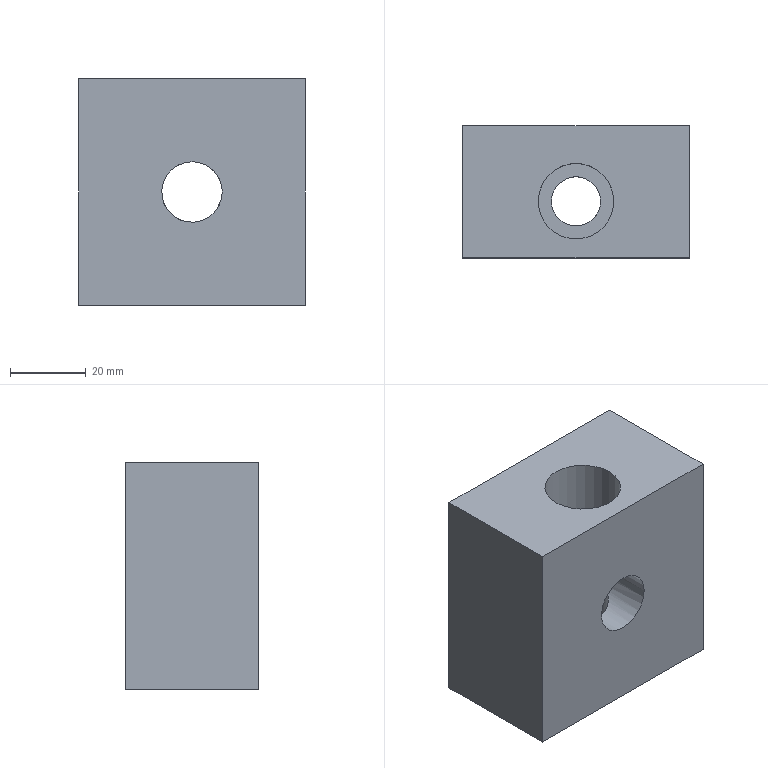Part | NX | features solid 2 | 1 solid | 11 faces | box 60 x 35 x 60 mm | volume 109054 mm3 | plane 7 | cylinder 4 | commonest cylinder face diameters 13 x1 13.5 x1 16 x1 20 x1
STEP:
#1=CARTESIAN_POINT('',(-250.,660.,-350.));
#2=VERTEX_POINT('',#1);
#3=CARTESIAN_POINT('',(-250.,695.,-350.));
#4=VERTEX_POINT('',#3);
#5=CARTESIAN_POINT('',(-250.,660.,-350.));
#6=DIRECTION('',(0.,1.,0.));
#7=VECTOR('',#6,1000.);
#8=LINE('',#5,#7);
#9=EDGE_CURVE('',#2,#4,#8,.T.);
#10=ORIENTED_EDGE('',*,*,#9,.T.);
#11=CARTESIAN_POINT('',(-310.,695.,-350.));
#12=VERTEX_POINT('',#11);
#13=CARTESIAN_POINT('',(-250.,695.,-350.));
#14=DIRECTION('',(-1.,0.,0.));
#15=VECTOR('',#14,1000.);
#16=LINE('',#13,#15);
#17=EDGE_CURVE('',#4,#12,#16,.T.);
#18=ORIENTED_EDGE('',*,*,#17,.T.);
#19=CARTESIAN_POINT('',(-310.,660.,-350.));
#20=VERTEX_POINT('',#19);
#21=CARTESIAN_POINT('',(-310.,660.,-350.));
#22=DIRECTION('',(0.,1.,0.));
#23=VECTOR('',#22,1000.);
#24=LINE('',#21,#23);
#25=EDGE_CURVE('',#20,#12,#24,.T.);
#26=ORIENTED_EDGE('',*,*,#25,.F.);
#27=CARTESIAN_POINT('',(-250.,660.,-350.));
#28=DIRECTION('',(-1.,0.,0.));
#29=VECTOR('',#28,1000.);
#30=LINE('',#27,#29);
#31=EDGE_CURVE('',#2,#20,#30,.T.);
#32=ORIENTED_EDGE('',*,*,#31,.F.);
#33=EDGE_LOOP('',(#10,#18,#26,#32));
#34=FACE_BOUND('',#33,.T.);
#35=CARTESIAN_POINT('',(-270.,675.,-350.));
#36=VERTEX_POINT('',#35);
#37=CARTESIAN_POINT('',(-280.,675.,-350.));
#38=DIRECTION('',(0.,0.,-1.));
#39=DIRECTION('',(1.,0.,0.));
#40=AXIS2_PLACEMENT_3D('',#37,#38,#39);
#41=CIRCLE('',#40,10.);
#42=EDGE_CURVE('',#36,#36,#41,.F.);
#43=ORIENTED_EDGE('',*,*,#42,.F.);
#44=EDGE_LOOP('',(#43));
#45=FACE_BOUND('',#44,.T.);
#46=CARTESIAN_POINT('',(-250.,660.,-350.));
#47=DIRECTION('',(0.,0.,-1.));
#48=DIRECTION('',(0.,1.,0.));
#49=AXIS2_PLACEMENT_3D('',#46,#47,#48);
#50=PLANE('',#49);
#51=ADVANCED_FACE('',(#34,#45),#50,.F.);
#52=CARTESIAN_POINT('',(-286.75,675.,-410.));
#53=VERTEX_POINT('',#52);
#54=CARTESIAN_POINT('',(-280.,675.,-410.));
#55=DIRECTION('',(0.,0.,1.));
#56=DIRECTION('',(-1.,0.,0.));
#57=AXIS2_PLACEMENT_3D('',#54,#55,#56);
#58=CIRCLE('',#57,6.75);
#59=EDGE_CURVE('',#53,#53,#58,.T.);
#60=ORIENTED_EDGE('',*,*,#59,.T.);
#61=EDGE_LOOP('',(#60));
#62=FACE_BOUND('',#61,.T.);
#63=CARTESIAN_POINT('',(-250.,695.,-410.));
#64=VERTEX_POINT('',#63);
#65=CARTESIAN_POINT('',(-310.,695.,-410.));
#66=VERTEX_POINT('',#65);
#67=CARTESIAN_POINT('',(-250.,695.,-410.));
#68=DIRECTION('',(-1.,0.,0.));
#69=VECTOR('',#68,1000.);
#70=LINE('',#67,#69);
#71=EDGE_CURVE('',#64,#66,#70,.T.);
#72=ORIENTED_EDGE('',*,*,#71,.F.);
#73=CARTESIAN_POINT('',(-250.,660.,-410.));
#74=VERTEX_POINT('',#73);
#75=CARTESIAN_POINT('',(-250.,660.,-410.));
#76=DIRECTION('',(0.,1.,0.));
#77=VECTOR('',#76,1000.);
#78=LINE('',#75,#77);
#79=EDGE_CURVE('',#74,#64,#78,.T.);
#80=ORIENTED_EDGE('',*,*,#79,.F.);
#81=CARTESIAN_POINT('',(-310.,660.,-410.));
#82=VERTEX_POINT('',#81);
#83=CARTESIAN_POINT('',(-310.,660.,-410.));
#84=DIRECTION('',(1.,0.,0.));
#85=VECTOR('',#84,1000.);
#86=LINE('',#83,#85);
#87=EDGE_CURVE('',#82,#74,#86,.T.);
#88=ORIENTED_EDGE('',*,*,#87,.F.);
#89=CARTESIAN_POINT('',(-310.,660.,-410.));
#90=DIRECTION('',(0.,1.,0.));
#91=VECTOR('',#90,1000.);
#92=LINE('',#89,#91);
#93=EDGE_CURVE('',#82,#66,#92,.T.);
#94=ORIENTED_EDGE('',*,*,#93,.T.);
#95=EDGE_LOOP('',(#72,#80,#88,#94));
#96=FACE_BOUND('',#95,.T.);
#97=CARTESIAN_POINT('',(-310.,660.,-410.));
#98=DIRECTION('',(0.,0.,1.));
#99=DIRECTION('',(0.,-1.,0.));
#100=AXIS2_PLACEMENT_3D('',#97,#98,#99);
#101=PLANE('',#100);
#102=ADVANCED_FACE('',(#62,#96),#101,.F.);
#103=ORIENTED_EDGE('',*,*,#9,.F.);
#104=CARTESIAN_POINT('',(-250.,660.,-410.));
#105=DIRECTION('',(0.,0.,1.));
#106=VECTOR('',#105,1000.);
#107=LINE('',#104,#106);
#108=EDGE_CURVE('',#74,#2,#107,.T.);
#109=ORIENTED_EDGE('',*,*,#108,.F.);
#110=ORIENTED_EDGE('',*,*,#79,.T.);
#111=CARTESIAN_POINT('',(-250.,695.,-410.));
#112=DIRECTION('',(0.,0.,-1.));
#113=VECTOR('',#112,1000.);
#114=LINE('',#111,#113);
#115=EDGE_CURVE('',#4,#64,#114,.T.);
#116=ORIENTED_EDGE('',*,*,#115,.F.);
#117=EDGE_LOOP('',(#103,#109,#110,#116));
#118=FACE_BOUND('',#117,.T.);
#119=CARTESIAN_POINT('',(-250.,660.,-410.));
#120=DIRECTION('',(-1.,0.,0.));
#121=DIRECTION('',(0.,-1.,0.));
#122=AXIS2_PLACEMENT_3D('',#119,#120,#121);
#123=PLANE('',#122);
#124=ADVANCED_FACE('',(#118),#123,.F.);
#125=CARTESIAN_POINT('',(-286.75,675.,-384.294));
#126=VERTEX_POINT('',#125);
#127=CARTESIAN_POINT('',(-286.336,677.772,-384.975));
#128=CARTESIAN_POINT('',(-286.957,674.999,-383.954));
#129=CARTESIAN_POINT('',(-286.337,672.233,-384.973));
#130=CARTESIAN_POINT('',(-284.957,670.207,-386.409));
#131=CARTESIAN_POINT('',(-282.834,668.669,-387.64));
#132=CARTESIAN_POINT('',(-280.007,668.042,-388.179));
#133=CARTESIAN_POINT('',(-277.175,668.664,-387.644));
#134=CARTESIAN_POINT('',(-275.046,670.204,-386.412));
#135=CARTESIAN_POINT('',(-273.663,672.229,-384.974));
#136=CARTESIAN_POINT('',(-273.043,675.006,-383.954));
#137=CARTESIAN_POINT('',(-273.663,677.771,-384.975));
#138=CARTESIAN_POINT('',(-275.05,679.8,-386.414));
#139=CARTESIAN_POINT('',(-277.163,681.328,-387.638));
#140=CARTESIAN_POINT('',(-279.987,681.959,-388.18));
#141=CARTESIAN_POINT('',(-282.827,681.336,-387.644));
#142=CARTESIAN_POINT('',(-284.953,679.797,-386.412));
#143=CARTESIAN_POINT('',(-286.336,677.772,-384.975));
#144=CARTESIAN_POINT('',(-286.957,674.999,-383.954));
#145=CARTESIAN_POINT('',(-286.337,672.233,-384.973));
#146=B_SPLINE_CURVE_WITH_KNOTS('',3,(#127,#128,#129,#130,#131,#132,#133,#134,#135,#136,#137,#138,#139,#140,#141,#142,#143,#144,#145),.UNSPECIFIED.,.T.,.F.,(1,1,1,1,1,1,1,1,1,1,1,1,1,1,1,1,1,1,1,1,1,1,1),(-0.008494,-0.005663,-0.002831,0.,0.002831,0.005663,0.008494,0.01133,0.01416,0.01699,0.01982,0.02265,0.02548,0.02831,0.03114,0.03398,0.03681,0.03964,0.04247,0.0453,0.04813,0.05096,0.05379),.UNSPECIFIED.);
#147=EDGE_CURVE('',#126,#126,#146,.T.);
#148=ORIENTED_EDGE('',*,*,#147,.F.);
#149=EDGE_LOOP('',(#148));
#150=FACE_BOUND('',#149,.T.);
#151=CARTESIAN_POINT('',(-273.511,675.371,-375.322));
#152=VERTEX_POINT('',#151);
#153=CARTESIAN_POINT('',(-274.043,677.97,-374.574));
#154=CARTESIAN_POINT('',(-273.316,675.398,-375.603));
#155=CARTESIAN_POINT('',(-273.755,672.661,-374.941));
#156=CARTESIAN_POINT('',(-275.015,670.616,-373.631));
#157=CARTESIAN_POINT('',(-276.942,669.071,-372.47));
#158=CARTESIAN_POINT('',(-279.577,668.317,-371.849));
#159=CARTESIAN_POINT('',(-282.323,668.735,-372.196));
#160=CARTESIAN_POINT('',(-284.497,670.104,-373.266));
#161=CARTESIAN_POINT('',(-285.942,672.008,-374.557));
#162=CARTESIAN_POINT('',(-286.68,674.546,-375.597));
#163=CARTESIAN_POINT('',(-286.258,677.311,-374.96));
#164=CARTESIAN_POINT('',(-285.,679.367,-373.643));
#165=CARTESIAN_POINT('',(-283.074,680.922,-372.476));
#166=CARTESIAN_POINT('',(-280.429,681.684,-371.848));
#167=CARTESIAN_POINT('',(-277.671,681.264,-372.197));
#168=CARTESIAN_POINT('',(-275.491,679.886,-373.272));
#169=CARTESIAN_POINT('',(-274.043,677.97,-374.574));
#170=CARTESIAN_POINT('',(-273.316,675.398,-375.603));
#171=CARTESIAN_POINT('',(-273.755,672.661,-374.941));
#172=B_SPLINE_CURVE_WITH_KNOTS('',3,(#153,#154,#155,#156,#157,#158,#159,#160,#161,#162,#163,#164,#165,#166,#167,#168,#169,#170,#171),.UNSPECIFIED.,.T.,.F.,(1,1,1,1,1,1,1,1,1,1,1,1,1,1,1,1,1,1,1,1,1,1,1),(-0.008099,-0.005399,-0.0027,0.,0.0027,0.005399,0.008099,0.0108,0.0135,0.0162,0.0189,0.0216,0.0243,0.027,0.0297,0.0324,0.0351,0.0378,0.0405,0.0432,0.04589,0.04859,0.05129),.UNSPECIFIED.);
#173=EDGE_CURVE('',#152,#152,#172,.T.);
#174=ORIENTED_EDGE('',*,*,#173,.F.);
#175=EDGE_LOOP('',(#174));
#176=FACE_BOUND('',#175,.T.);
#177=CARTESIAN_POINT('',(-272.,660.,-380.));
#178=VERTEX_POINT('',#177);
#179=CARTESIAN_POINT('',(-280.,660.,-380.));
#180=DIRECTION('',(0.,-1.,0.));
#181=DIRECTION('',(1.,0.,0.));
#182=AXIS2_PLACEMENT_3D('',#179,#180,#181);
#183=CIRCLE('',#182,8.);
#184=EDGE_CURVE('',#178,#178,#183,.T.);
#185=ORIENTED_EDGE('',*,*,#184,.T.);
#186=EDGE_LOOP('',(#185));
#187=FACE_BOUND('',#186,.T.);
#188=CARTESIAN_POINT('',(-280.,695.,-372.));
#189=VERTEX_POINT('',#188);
#190=CARTESIAN_POINT('',(-280.,695.,-380.));
#191=DIRECTION('',(0.,-1.,0.));
#192=DIRECTION('',(0.,0.,1.));
#193=AXIS2_PLACEMENT_3D('',#190,#191,#192);
#194=CIRCLE('',#193,8.);
#195=EDGE_CURVE('',#189,#189,#194,.T.);
#196=ORIENTED_EDGE('',*,*,#195,.F.);
#197=EDGE_LOOP('',(#196));
#198=FACE_BOUND('',#197,.T.);
#199=CARTESIAN_POINT('',(-280.,660.,-380.));
#200=DIRECTION('',(0.,1.,0.));
#201=DIRECTION('',(-1.,0.,0.));
#202=AXIS2_PLACEMENT_3D('',#199,#200,#201);
#203=CYLINDRICAL_SURFACE('',#202,8.);
#204=ADVANCED_FACE('',(#150,#176,#187,#198),#203,.F.);
#205=CARTESIAN_POINT('',(-310.,660.,-410.));
#206=DIRECTION('',(0.,0.,1.));
#207=VECTOR('',#206,1000.);
#208=LINE('',#205,#207);
#209=EDGE_CURVE('',#82,#20,#208,.T.);
#210=ORIENTED_EDGE('',*,*,#209,.T.);
#211=ORIENTED_EDGE('',*,*,#25,.T.);
#212=CARTESIAN_POINT('',(-310.,695.,-350.));
#213=DIRECTION('',(0.,0.,-1.));
#214=VECTOR('',#213,1000.);
#215=LINE('',#212,#214);
#216=EDGE_CURVE('',#12,#66,#215,.T.);
#217=ORIENTED_EDGE('',*,*,#216,.T.);
#218=ORIENTED_EDGE('',*,*,#93,.F.);
#219=EDGE_LOOP('',(#210,#211,#217,#218));
#220=FACE_BOUND('',#219,.T.);
#221=CARTESIAN_POINT('',(-310.,660.,-350.));
#222=DIRECTION('',(1.,0.,0.));
#223=DIRECTION('',(0.,1.,0.));
#224=AXIS2_PLACEMENT_3D('',#221,#222,#223);
#225=PLANE('',#224);
#226=ADVANCED_FACE('',(#220),#225,.F.);
#227=ORIENTED_EDGE('',*,*,#108,.T.);
#228=ORIENTED_EDGE('',*,*,#31,.T.);
#229=ORIENTED_EDGE('',*,*,#209,.F.);
#230=ORIENTED_EDGE('',*,*,#87,.T.);
#231=EDGE_LOOP('',(#227,#228,#229,#230));
#232=FACE_BOUND('',#231,.T.);
#233=ORIENTED_EDGE('',*,*,#184,.F.);
#234=EDGE_LOOP('',(#233));
#235=FACE_BOUND('',#234,.T.);
#236=CARTESIAN_POINT('',(-250.,660.,-410.));
#237=DIRECTION('',(0.,-1.,0.));
#238=DIRECTION('',(1.,0.,0.));
#239=AXIS2_PLACEMENT_3D('',#236,#237,#238);
#240=PLANE('',#239);
#241=ADVANCED_FACE('',(#232,#235),#240,.T.);
#242=ORIENTED_EDGE('',*,*,#17,.F.);
#243=ORIENTED_EDGE('',*,*,#115,.T.);
#244=ORIENTED_EDGE('',*,*,#71,.T.);
#245=ORIENTED_EDGE('',*,*,#216,.F.);
#246=EDGE_LOOP('',(#242,#243,#244,#245));
#247=FACE_BOUND('',#246,.T.);
#248=ORIENTED_EDGE('',*,*,#195,.T.);
#249=EDGE_LOOP('',(#248));
#250=FACE_BOUND('',#249,.T.);
#251=CARTESIAN_POINT('',(-250.,695.,-410.));
#252=DIRECTION('',(0.,-1.,0.));
#253=DIRECTION('',(1.,0.,0.));
#254=AXIS2_PLACEMENT_3D('',#251,#252,#253);
#255=PLANE('',#254);
#256=ADVANCED_FACE('',(#247,#250),#255,.F.);
#257=CARTESIAN_POINT('',(-290.,675.,-370.));
#258=VERTEX_POINT('',#257);
#259=CARTESIAN_POINT('',(-280.,675.,-370.));
#260=DIRECTION('',(0.,0.,1.));
#261=DIRECTION('',(-1.,0.,0.));
#262=AXIS2_PLACEMENT_3D('',#259,#260,#261);
#263=CIRCLE('',#262,10.);
#264=EDGE_CURVE('',#258,#258,#263,.T.);
#265=ORIENTED_EDGE('',*,*,#264,.F.);
#266=EDGE_LOOP('',(#265));
#267=FACE_BOUND('',#266,.T.);
#268=ORIENTED_EDGE('',*,*,#42,.T.);
#269=EDGE_LOOP('',(#268));
#270=FACE_BOUND('',#269,.T.);
#271=CARTESIAN_POINT('',(-280.,675.,-320.));
#272=DIRECTION('',(0.,0.,-1.));
#273=DIRECTION('',(1.,0.,0.));
#274=AXIS2_PLACEMENT_3D('',#271,#272,#273);
#275=CYLINDRICAL_SURFACE('',#274,10.);
#276=ADVANCED_FACE('',(#267,#270),#275,.F.);
#277=CARTESIAN_POINT('',(-286.5,675.,-370.));
#278=VERTEX_POINT('',#277);
#279=CARTESIAN_POINT('',(-280.,675.,-370.));
#280=DIRECTION('',(0.,0.,1.));
#281=DIRECTION('',(-1.,0.,0.));
#282=AXIS2_PLACEMENT_3D('',#279,#280,#281);
#283=CIRCLE('',#282,6.5);
#284=EDGE_CURVE('',#278,#278,#283,.T.);
#285=ORIENTED_EDGE('',*,*,#284,.F.);
#286=EDGE_LOOP('',(#285));
#287=FACE_BOUND('',#286,.T.);
#288=ORIENTED_EDGE('',*,*,#264,.T.);
#289=EDGE_LOOP('',(#288));
#290=FACE_BOUND('',#289,.T.);
#291=CARTESIAN_POINT('',(-280.,675.,-370.));
#292=DIRECTION('',(0.,0.,1.));
#293=DIRECTION('',(-1.,0.,0.));
#294=AXIS2_PLACEMENT_3D('',#291,#292,#293);
#295=PLANE('',#294);
#296=ADVANCED_FACE('',(#287,#290),#295,.T.);
#297=ORIENTED_EDGE('',*,*,#173,.T.);
#298=EDGE_LOOP('',(#297));
#299=FACE_BOUND('',#298,.T.);
#300=ORIENTED_EDGE('',*,*,#284,.T.);
#301=EDGE_LOOP('',(#300));
#302=FACE_BOUND('',#301,.T.);
#303=CARTESIAN_POINT('',(-280.,675.,-420.));
#304=DIRECTION('',(0.,0.,1.));
#305=DIRECTION('',(-1.,0.,0.));
#306=AXIS2_PLACEMENT_3D('',#303,#304,#305);
#307=CYLINDRICAL_SURFACE('',#306,6.5);
#308=ADVANCED_FACE('',(#299,#302),#307,.F.);
#309=ORIENTED_EDGE('',*,*,#147,.T.);
#310=EDGE_LOOP('',(#309));
#311=FACE_BOUND('',#310,.T.);
#312=ORIENTED_EDGE('',*,*,#59,.F.);
#313=EDGE_LOOP('',(#312));
#314=FACE_BOUND('',#313,.T.);
#315=CARTESIAN_POINT('',(-280.,675.,-420.));
#316=DIRECTION('',(0.,0.,1.));
#317=DIRECTION('',(-1.,0.,0.));
#318=AXIS2_PLACEMENT_3D('',#315,#316,#317);
#319=CYLINDRICAL_SURFACE('',#318,6.75);
#320=ADVANCED_FACE('',(#311,#314),#319,.F.);
#321=CLOSED_SHELL('',(#51,#102,#124,#204,#226,#241,#256,#276,#296,#308,#320));
#322=MANIFOLD_SOLID_BREP('',#321);
#323=(LENGTH_UNIT()NAMED_UNIT(*)SI_UNIT(.MILLI.,.METRE.));
#324=UNCERTAINTY_MEASURE_WITH_UNIT(LENGTH_MEASURE(0.0508),#323,'','');
#325=(NAMED_UNIT(*)PLANE_ANGLE_UNIT()SI_UNIT($,.RADIAN.));
#326=(NAMED_UNIT(*)SI_UNIT($,.STERADIAN.)SOLID_ANGLE_UNIT());
#327=(GEOMETRIC_REPRESENTATION_CONTEXT(3)GLOBAL_UNCERTAINTY_ASSIGNED_CONTEXT((#324))GLOBAL_UNIT_ASSIGNED_CONTEXT((#323,#325,#326))REPRESENTATION_CONTEXT('',''));
#328=ADVANCED_BREP_SHAPE_REPRESENTATION('',(#322),#327);